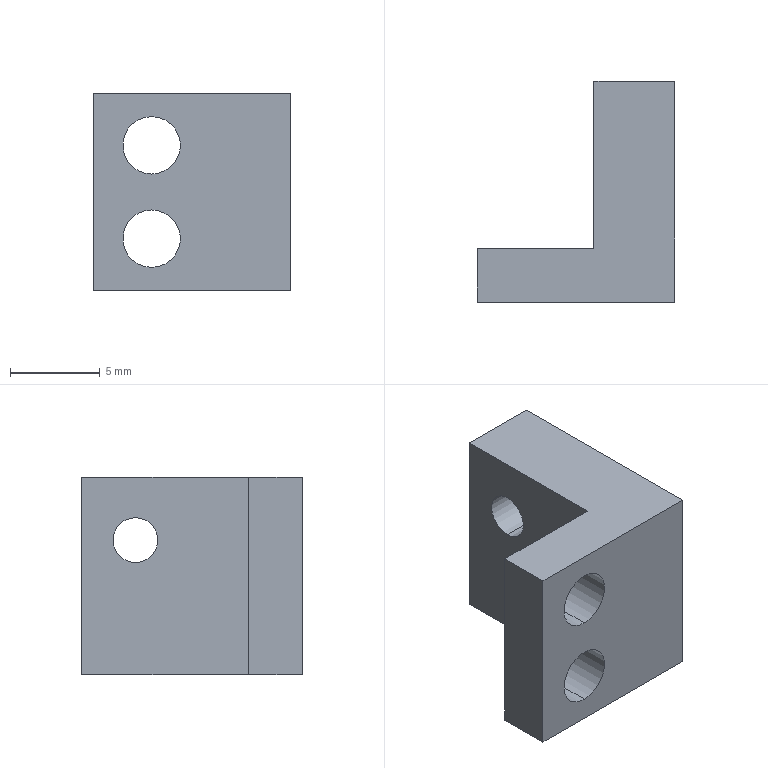Part | SolidWorks | features ICE 2, Chamfer 1, Extrusion 1, HoleWzd 1 | 1 solid | 18 faces | box 11 x 12.3 x 11 mm | volume 750.231 mm3 | plane 8 | cylinder 6 | cone 4 | commonest cylinder face diameters 3.2 x4 2.5 x2
STEP:
#1=CARTESIAN_POINT('',(-2.25,2.5,-4.2));
#2=VERTEX_POINT('',#1);
#3=CARTESIAN_POINT('',(-2.25,2.5,-1.));
#4=VERTEX_POINT('',#3);
#5=CARTESIAN_POINT('',(-2.25,2.5,-2.6));
#6=DIRECTION('',(0.,1.,0.));
#7=DIRECTION('',(0.,0.,1.));
#8=AXIS2_PLACEMENT_3D('',#5,#6,#7);
#9=CIRCLE('',#8,1.6);
#10=EDGE_CURVE('',#2,#4,#9,.T.);
#11=ORIENTED_EDGE('',*,*,#10,.F.);
#12=CARTESIAN_POINT('',(-2.25,3.,-4.7));
#13=VERTEX_POINT('',#12);
#14=CARTESIAN_POINT('',(-2.25,2.5,-4.2));
#15=DIRECTION('',(0.,0.7071,-0.7071));
#16=VECTOR('',#15,1000.);
#17=LINE('',#14,#16);
#18=EDGE_CURVE('',#2,#13,#17,.T.);
#19=ORIENTED_EDGE('',*,*,#18,.T.);
#20=CARTESIAN_POINT('',(-2.25,3.,-0.5));
#21=VERTEX_POINT('',#20);
#22=CARTESIAN_POINT('',(-2.25,3.,-2.6));
#23=DIRECTION('',(0.,-1.,0.));
#24=DIRECTION('',(0.,0.,1.));
#25=AXIS2_PLACEMENT_3D('',#22,#23,#24);
#26=CIRCLE('',#25,2.1);
#27=EDGE_CURVE('',#21,#13,#26,.T.);
#28=ORIENTED_EDGE('',*,*,#27,.F.);
#29=CARTESIAN_POINT('',(-2.25,2.5,-1.));
#30=DIRECTION('',(0.,0.7071,0.7071));
#31=VECTOR('',#30,1000.);
#32=LINE('',#29,#31);
#33=EDGE_CURVE('',#4,#21,#32,.T.);
#34=ORIENTED_EDGE('',*,*,#33,.F.);
#35=EDGE_LOOP('',(#11,#19,#28,#34));
#36=FACE_OUTER_BOUND('',#35,.T.);
#37=CARTESIAN_POINT('',(-2.25,2.5,-2.6));
#38=DIRECTION('',(0.,1.,0.));
#39=DIRECTION('',(0.,0.,1.));
#40=AXIS2_PLACEMENT_3D('',#37,#38,#39);
#41=CONICAL_SURFACE('',#40,1.6,0.7854);
#42=ADVANCED_FACE('',(#36),#41,.F.);
#43=CARTESIAN_POINT('',(-2.25,2.5,1.));
#44=VERTEX_POINT('',#43);
#45=CARTESIAN_POINT('',(-2.25,2.5,4.2));
#46=VERTEX_POINT('',#45);
#47=CARTESIAN_POINT('',(-2.25,2.5,2.6));
#48=DIRECTION('',(0.,1.,0.));
#49=DIRECTION('',(0.,0.,1.));
#50=AXIS2_PLACEMENT_3D('',#47,#48,#49);
#51=CIRCLE('',#50,1.6);
#52=EDGE_CURVE('',#44,#46,#51,.T.);
#53=ORIENTED_EDGE('',*,*,#52,.F.);
#54=CARTESIAN_POINT('',(-2.25,3.,0.5));
#55=VERTEX_POINT('',#54);
#56=CARTESIAN_POINT('',(-2.25,2.5,1.));
#57=DIRECTION('',(0.,0.7071,-0.7071));
#58=VECTOR('',#57,1000.);
#59=LINE('',#56,#58);
#60=EDGE_CURVE('',#44,#55,#59,.T.);
#61=ORIENTED_EDGE('',*,*,#60,.T.);
#62=CARTESIAN_POINT('',(-2.25,3.,4.7));
#63=VERTEX_POINT('',#62);
#64=CARTESIAN_POINT('',(-2.25,3.,2.6));
#65=DIRECTION('',(0.,-1.,0.));
#66=DIRECTION('',(0.,0.,1.));
#67=AXIS2_PLACEMENT_3D('',#64,#65,#66);
#68=CIRCLE('',#67,2.1);
#69=EDGE_CURVE('',#63,#55,#68,.T.);
#70=ORIENTED_EDGE('',*,*,#69,.F.);
#71=CARTESIAN_POINT('',(-2.25,2.5,4.2));
#72=DIRECTION('',(0.,0.7071,0.7071));
#73=VECTOR('',#72,1000.);
#74=LINE('',#71,#73);
#75=EDGE_CURVE('',#46,#63,#74,.T.);
#76=ORIENTED_EDGE('',*,*,#75,.F.);
#77=EDGE_LOOP('',(#53,#61,#70,#76));
#78=FACE_OUTER_BOUND('',#77,.T.);
#79=CARTESIAN_POINT('',(-2.25,2.5,2.6));
#80=DIRECTION('',(0.,1.,0.));
#81=DIRECTION('',(0.,0.,1.));
#82=AXIS2_PLACEMENT_3D('',#79,#80,#81);
#83=CONICAL_SURFACE('',#82,1.6,0.7854);
#84=ADVANCED_FACE('',(#78),#83,.F.);
#85=CARTESIAN_POINT('',(-2.25,0.,-4.2));
#86=VERTEX_POINT('',#85);
#87=CARTESIAN_POINT('',(-2.25,0.,-1.));
#88=VERTEX_POINT('',#87);
#89=CARTESIAN_POINT('',(-2.25,0.,-2.6));
#90=DIRECTION('',(0.,1.,0.));
#91=DIRECTION('',(0.,0.,1.));
#92=AXIS2_PLACEMENT_3D('',#89,#90,#91);
#93=CIRCLE('',#92,1.6);
#94=EDGE_CURVE('',#86,#88,#93,.T.);
#95=ORIENTED_EDGE('',*,*,#94,.F.);
#96=CARTESIAN_POINT('',(-2.25,0.,-4.2));
#97=DIRECTION('',(0.,1.,0.));
#98=VECTOR('',#97,1000.);
#99=LINE('',#96,#98);
#100=EDGE_CURVE('',#86,#2,#99,.T.);
#101=ORIENTED_EDGE('',*,*,#100,.T.);
#102=ORIENTED_EDGE('',*,*,#10,.T.);
#103=CARTESIAN_POINT('',(-2.25,0.,-1.));
#104=DIRECTION('',(0.,1.,0.));
#105=VECTOR('',#104,1000.);
#106=LINE('',#103,#105);
#107=EDGE_CURVE('',#88,#4,#106,.T.);
#108=ORIENTED_EDGE('',*,*,#107,.F.);
#109=EDGE_LOOP('',(#95,#101,#102,#108));
#110=FACE_OUTER_BOUND('',#109,.T.);
#111=CARTESIAN_POINT('',(-2.25,0.,-2.6));
#112=DIRECTION('',(0.,1.,0.));
#113=DIRECTION('',(0.,0.,1.));
#114=AXIS2_PLACEMENT_3D('',#111,#112,#113);
#115=CYLINDRICAL_SURFACE('',#114,1.6);
#116=ADVANCED_FACE('',(#110),#115,.F.);
#117=CARTESIAN_POINT('',(-2.25,0.,1.));
#118=VERTEX_POINT('',#117);
#119=CARTESIAN_POINT('',(-2.25,0.,4.2));
#120=VERTEX_POINT('',#119);
#121=CARTESIAN_POINT('',(-2.25,0.,2.6));
#122=DIRECTION('',(0.,1.,0.));
#123=DIRECTION('',(0.,0.,1.));
#124=AXIS2_PLACEMENT_3D('',#121,#122,#123);
#125=CIRCLE('',#124,1.6);
#126=EDGE_CURVE('',#118,#120,#125,.T.);
#127=ORIENTED_EDGE('',*,*,#126,.F.);
#128=CARTESIAN_POINT('',(-2.25,0.,1.));
#129=DIRECTION('',(0.,1.,0.));
#130=VECTOR('',#129,1000.);
#131=LINE('',#128,#130);
#132=EDGE_CURVE('',#118,#44,#131,.T.);
#133=ORIENTED_EDGE('',*,*,#132,.T.);
#134=ORIENTED_EDGE('',*,*,#52,.T.);
#135=CARTESIAN_POINT('',(-2.25,0.,4.2));
#136=DIRECTION('',(0.,1.,0.));
#137=VECTOR('',#136,1000.);
#138=LINE('',#135,#137);
#139=EDGE_CURVE('',#120,#46,#138,.T.);
#140=ORIENTED_EDGE('',*,*,#139,.F.);
#141=EDGE_LOOP('',(#127,#133,#134,#140));
#142=FACE_OUTER_BOUND('',#141,.T.);
#143=CARTESIAN_POINT('',(-2.25,0.,2.6));
#144=DIRECTION('',(0.,1.,0.));
#145=DIRECTION('',(0.,0.,1.));
#146=AXIS2_PLACEMENT_3D('',#143,#144,#145);
#147=CYLINDRICAL_SURFACE('',#146,1.6);
#148=ADVANCED_FACE('',(#142),#147,.F.);
#149=CARTESIAN_POINT('',(5.5,9.3,0.75));
#150=VERTEX_POINT('',#149);
#151=CARTESIAN_POINT('',(5.5,9.3,3.25));
#152=VERTEX_POINT('',#151);
#153=CARTESIAN_POINT('',(5.5,9.3,2.));
#154=DIRECTION('',(-1.,0.,0.));
#155=DIRECTION('',(0.,0.,1.));
#156=AXIS2_PLACEMENT_3D('',#153,#154,#155);
#157=CIRCLE('',#156,1.25);
#158=EDGE_CURVE('',#150,#152,#157,.T.);
#159=ORIENTED_EDGE('',*,*,#158,.F.);
#160=CARTESIAN_POINT('',(1.,9.3,0.75));
#161=VERTEX_POINT('',#160);
#162=CARTESIAN_POINT('',(1.,9.3,0.75));
#163=DIRECTION('',(-1.,0.,0.));
#164=VECTOR('',#163,1000.);
#165=LINE('',#162,#164);
#166=EDGE_CURVE('',#150,#161,#165,.T.);
#167=ORIENTED_EDGE('',*,*,#166,.T.);
#168=CARTESIAN_POINT('',(1.,9.3,3.25));
#169=VERTEX_POINT('',#168);
#170=CARTESIAN_POINT('',(1.,9.3,2.));
#171=DIRECTION('',(-1.,0.,0.));
#172=DIRECTION('',(0.,0.,1.));
#173=AXIS2_PLACEMENT_3D('',#170,#171,#172);
#174=CIRCLE('',#173,1.25);
#175=EDGE_CURVE('',#161,#169,#174,.T.);
#176=ORIENTED_EDGE('',*,*,#175,.T.);
#177=CARTESIAN_POINT('',(1.,9.3,3.25));
#178=DIRECTION('',(-1.,0.,0.));
#179=VECTOR('',#178,1000.);
#180=LINE('',#177,#179);
#181=EDGE_CURVE('',#152,#169,#180,.T.);
#182=ORIENTED_EDGE('',*,*,#181,.F.);
#183=EDGE_LOOP('',(#159,#167,#176,#182));
#184=FACE_OUTER_BOUND('',#183,.T.);
#185=CARTESIAN_POINT('',(1.,9.3,2.));
#186=DIRECTION('',(-1.,0.,0.));
#187=DIRECTION('',(0.,0.,1.));
#188=AXIS2_PLACEMENT_3D('',#185,#186,#187);
#189=CYLINDRICAL_SURFACE('',#188,1.25);
#190=ADVANCED_FACE('',(#184),#189,.F.);
#191=CARTESIAN_POINT('',(5.5,9.3,2.));
#192=DIRECTION('',(-1.,0.,0.));
#193=DIRECTION('',(0.,0.,1.));
#194=AXIS2_PLACEMENT_3D('',#191,#192,#193);
#195=CIRCLE('',#194,1.25);
#196=EDGE_CURVE('',#152,#150,#195,.T.);
#197=ORIENTED_EDGE('',*,*,#196,.T.);
#198=ORIENTED_EDGE('',*,*,#158,.T.);
#199=EDGE_LOOP('',(#197,#198));
#200=FACE_BOUND('',#199,.T.);
#201=CARTESIAN_POINT('',(5.5,0.,5.5));
#202=VERTEX_POINT('',#201);
#203=CARTESIAN_POINT('',(5.5,0.,-5.5));
#204=VERTEX_POINT('',#203);
#205=CARTESIAN_POINT('',(5.5,0.,-5.5));
#206=DIRECTION('',(0.,0.,-1.));
#207=VECTOR('',#206,1000.);
#208=LINE('',#205,#207);
#209=EDGE_CURVE('',#202,#204,#208,.T.);
#210=ORIENTED_EDGE('',*,*,#209,.T.);
#211=CARTESIAN_POINT('',(5.5,12.3,-5.5));
#212=VERTEX_POINT('',#211);
#213=CARTESIAN_POINT('',(5.5,3.,-5.5));
#214=DIRECTION('',(0.,-1.,0.));
#215=VECTOR('',#214,1000.);
#216=LINE('',#213,#215);
#217=EDGE_CURVE('',#212,#204,#216,.T.);
#218=ORIENTED_EDGE('',*,*,#217,.F.);
#219=CARTESIAN_POINT('',(5.5,12.3,5.5));
#220=VERTEX_POINT('',#219);
#221=CARTESIAN_POINT('',(5.5,12.3,-5.5));
#222=DIRECTION('',(0.,0.,-1.));
#223=VECTOR('',#222,1000.);
#224=LINE('',#221,#223);
#225=EDGE_CURVE('',#220,#212,#224,.T.);
#226=ORIENTED_EDGE('',*,*,#225,.F.);
#227=CARTESIAN_POINT('',(5.5,3.,5.5));
#228=DIRECTION('',(0.,-1.,0.));
#229=VECTOR('',#228,1000.);
#230=LINE('',#227,#229);
#231=EDGE_CURVE('',#220,#202,#230,.T.);
#232=ORIENTED_EDGE('',*,*,#231,.T.);
#233=EDGE_LOOP('',(#210,#218,#226,#232));
#234=FACE_OUTER_BOUND('',#233,.T.);
#235=CARTESIAN_POINT('',(5.5,3.,-5.5));
#236=DIRECTION('',(-1.,0.,0.));
#237=DIRECTION('',(0.,0.,1.));
#238=AXIS2_PLACEMENT_3D('',#235,#236,#237);
#239=PLANE('',#238);
#240=ADVANCED_FACE('',(#200,#234),#239,.F.);
#241=CARTESIAN_POINT('',(-5.5,0.,-5.5));
#242=VERTEX_POINT('',#241);
#243=CARTESIAN_POINT('',(-5.5,0.,-5.5));
#244=DIRECTION('',(-1.,0.,0.));
#245=VECTOR('',#244,1000.);
#246=LINE('',#243,#245);
#247=EDGE_CURVE('',#204,#242,#246,.T.);
#248=ORIENTED_EDGE('',*,*,#247,.T.);
#249=CARTESIAN_POINT('',(-5.5,3.,-5.5));
#250=VERTEX_POINT('',#249);
#251=CARTESIAN_POINT('',(-5.5,3.,-5.5));
#252=DIRECTION('',(0.,-1.,0.));
#253=VECTOR('',#252,1000.);
#254=LINE('',#251,#253);
#255=EDGE_CURVE('',#250,#242,#254,.T.);
#256=ORIENTED_EDGE('',*,*,#255,.F.);
#257=CARTESIAN_POINT('',(1.,3.,-5.5));
#258=VERTEX_POINT('',#257);
#259=CARTESIAN_POINT('',(-5.5,3.,-5.5));
#260=DIRECTION('',(-1.,0.,0.));
#261=VECTOR('',#260,1000.);
#262=LINE('',#259,#261);
#263=EDGE_CURVE('',#258,#250,#262,.T.);
#264=ORIENTED_EDGE('',*,*,#263,.F.);
#265=CARTESIAN_POINT('',(1.,12.3,-5.5));
#266=VERTEX_POINT('',#265);
#267=CARTESIAN_POINT('',(1.,12.3,-5.5));
#268=DIRECTION('',(0.,-1.,0.));
#269=VECTOR('',#268,1000.);
#270=LINE('',#267,#269);
#271=EDGE_CURVE('',#266,#258,#270,.T.);
#272=ORIENTED_EDGE('',*,*,#271,.F.);
#273=CARTESIAN_POINT('',(5.5,12.3,-5.5));
#274=DIRECTION('',(-1.,0.,0.));
#275=VECTOR('',#274,1000.);
#276=LINE('',#273,#275);
#277=EDGE_CURVE('',#212,#266,#276,.T.);
#278=ORIENTED_EDGE('',*,*,#277,.F.);
#279=ORIENTED_EDGE('',*,*,#217,.T.);
#280=EDGE_LOOP('',(#248,#256,#264,#272,#278,#279));
#281=FACE_OUTER_BOUND('',#280,.T.);
#282=CARTESIAN_POINT('',(-5.5,3.,-5.5));
#283=DIRECTION('',(0.,0.,1.));
#284=DIRECTION('',(1.,0.,0.));
#285=AXIS2_PLACEMENT_3D('',#282,#283,#284);
#286=PLANE('',#285);
#287=ADVANCED_FACE('',(#281),#286,.F.);
#288=CARTESIAN_POINT('',(-5.5,0.,5.5));
#289=VERTEX_POINT('',#288);
#290=CARTESIAN_POINT('',(-5.5,0.,-5.5));
#291=DIRECTION('',(0.,0.,1.));
#292=VECTOR('',#291,1000.);
#293=LINE('',#290,#292);
#294=EDGE_CURVE('',#242,#289,#293,.T.);
#295=ORIENTED_EDGE('',*,*,#294,.T.);
#296=CARTESIAN_POINT('',(-5.5,3.,5.5));
#297=VERTEX_POINT('',#296);
#298=CARTESIAN_POINT('',(-5.5,3.,5.5));
#299=DIRECTION('',(0.,-1.,0.));
#300=VECTOR('',#299,1000.);
#301=LINE('',#298,#300);
#302=EDGE_CURVE('',#297,#289,#301,.T.);
#303=ORIENTED_EDGE('',*,*,#302,.F.);
#304=CARTESIAN_POINT('',(-5.5,3.,-5.5));
#305=DIRECTION('',(0.,0.,1.));
#306=VECTOR('',#305,1000.);
#307=LINE('',#304,#306);
#308=EDGE_CURVE('',#250,#297,#307,.T.);
#309=ORIENTED_EDGE('',*,*,#308,.F.);
#310=ORIENTED_EDGE('',*,*,#255,.T.);
#311=EDGE_LOOP('',(#295,#303,#309,#310));
#312=FACE_OUTER_BOUND('',#311,.T.);
#313=CARTESIAN_POINT('',(-5.5,3.,-5.5));
#314=DIRECTION('',(1.,0.,0.));
#315=DIRECTION('',(0.,0.,-1.));
#316=AXIS2_PLACEMENT_3D('',#313,#314,#315);
#317=PLANE('',#316);
#318=ADVANCED_FACE('',(#312),#317,.F.);
#319=CARTESIAN_POINT('',(-5.5,0.,5.5));
#320=DIRECTION('',(1.,0.,0.));
#321=VECTOR('',#320,1000.);
#322=LINE('',#319,#321);
#323=EDGE_CURVE('',#289,#202,#322,.T.);
#324=ORIENTED_EDGE('',*,*,#323,.T.);
#325=ORIENTED_EDGE('',*,*,#231,.F.);
#326=CARTESIAN_POINT('',(1.,12.3,5.5));
#327=VERTEX_POINT('',#326);
#328=CARTESIAN_POINT('',(5.5,12.3,5.5));
#329=DIRECTION('',(1.,0.,0.));
#330=VECTOR('',#329,1000.);
#331=LINE('',#328,#330);
#332=EDGE_CURVE('',#327,#220,#331,.T.);
#333=ORIENTED_EDGE('',*,*,#332,.F.);
#334=CARTESIAN_POINT('',(1.,3.,5.5));
#335=VERTEX_POINT('',#334);
#336=CARTESIAN_POINT('',(1.,12.3,5.5));
#337=DIRECTION('',(0.,-1.,0.));
#338=VECTOR('',#337,1000.);
#339=LINE('',#336,#338);
#340=EDGE_CURVE('',#327,#335,#339,.T.);
#341=ORIENTED_EDGE('',*,*,#340,.T.);
#342=CARTESIAN_POINT('',(-5.5,3.,5.5));
#343=DIRECTION('',(1.,0.,0.));
#344=VECTOR('',#343,1000.);
#345=LINE('',#342,#344);
#346=EDGE_CURVE('',#297,#335,#345,.T.);
#347=ORIENTED_EDGE('',*,*,#346,.F.);
#348=ORIENTED_EDGE('',*,*,#302,.T.);
#349=EDGE_LOOP('',(#324,#325,#333,#341,#347,#348));
#350=FACE_OUTER_BOUND('',#349,.T.);
#351=CARTESIAN_POINT('',(-5.5,3.,5.5));
#352=DIRECTION('',(0.,0.,-1.));
#353=DIRECTION('',(-1.,0.,0.));
#354=AXIS2_PLACEMENT_3D('',#351,#352,#353);
#355=PLANE('',#354);
#356=ADVANCED_FACE('',(#350),#355,.F.);
#357=ORIENTED_EDGE('',*,*,#69,.T.);
#358=CARTESIAN_POINT('',(-2.25,3.,2.6));
#359=DIRECTION('',(0.,-1.,0.));
#360=DIRECTION('',(0.,0.,1.));
#361=AXIS2_PLACEMENT_3D('',#358,#359,#360);
#362=CIRCLE('',#361,2.1);
#363=EDGE_CURVE('',#55,#63,#362,.T.);
#364=ORIENTED_EDGE('',*,*,#363,.T.);
#365=EDGE_LOOP('',(#357,#364));
#366=FACE_BOUND('',#365,.T.);
#367=ORIENTED_EDGE('',*,*,#27,.T.);
#368=CARTESIAN_POINT('',(-2.25,3.,-2.6));
#369=DIRECTION('',(0.,-1.,0.));
#370=DIRECTION('',(0.,0.,1.));
#371=AXIS2_PLACEMENT_3D('',#368,#369,#370);
#372=CIRCLE('',#371,2.1);
#373=EDGE_CURVE('',#13,#21,#372,.T.);
#374=ORIENTED_EDGE('',*,*,#373,.T.);
#375=EDGE_LOOP('',(#367,#374));
#376=FACE_BOUND('',#375,.T.);
#377=CARTESIAN_POINT('',(1.,3.,-5.5));
#378=DIRECTION('',(0.,0.,1.));
#379=VECTOR('',#378,1000.);
#380=LINE('',#377,#379);
#381=EDGE_CURVE('',#258,#335,#380,.T.);
#382=ORIENTED_EDGE('',*,*,#381,.F.);
#383=ORIENTED_EDGE('',*,*,#263,.T.);
#384=ORIENTED_EDGE('',*,*,#308,.T.);
#385=ORIENTED_EDGE('',*,*,#346,.T.);
#386=EDGE_LOOP('',(#382,#383,#384,#385));
#387=FACE_OUTER_BOUND('',#386,.T.);
#388=CARTESIAN_POINT('',(0.,3.,0.));
#389=DIRECTION('',(0.,1.,0.));
#390=DIRECTION('',(0.,0.,1.));
#391=AXIS2_PLACEMENT_3D('',#388,#389,#390);
#392=PLANE('',#391);
#393=ADVANCED_FACE('',(#366,#376,#387),#392,.T.);
#394=CARTESIAN_POINT('',(-2.25,0.,-2.6));
#395=DIRECTION('',(0.,1.,0.));
#396=DIRECTION('',(0.,0.,1.));
#397=AXIS2_PLACEMENT_3D('',#394,#395,#396);
#398=CIRCLE('',#397,1.6);
#399=EDGE_CURVE('',#88,#86,#398,.T.);
#400=ORIENTED_EDGE('',*,*,#399,.T.);
#401=ORIENTED_EDGE('',*,*,#94,.T.);
#402=EDGE_LOOP('',(#400,#401));
#403=FACE_BOUND('',#402,.T.);
#404=CARTESIAN_POINT('',(-2.25,0.,2.6));
#405=DIRECTION('',(0.,1.,0.));
#406=DIRECTION('',(0.,0.,1.));
#407=AXIS2_PLACEMENT_3D('',#404,#405,#406);
#408=CIRCLE('',#407,1.6);
#409=EDGE_CURVE('',#120,#118,#408,.T.);
#410=ORIENTED_EDGE('',*,*,#409,.T.);
#411=ORIENTED_EDGE('',*,*,#126,.T.);
#412=EDGE_LOOP('',(#410,#411));
#413=FACE_BOUND('',#412,.T.);
#414=ORIENTED_EDGE('',*,*,#209,.F.);
#415=ORIENTED_EDGE('',*,*,#323,.F.);
#416=ORIENTED_EDGE('',*,*,#294,.F.);
#417=ORIENTED_EDGE('',*,*,#247,.F.);
#418=EDGE_LOOP('',(#414,#415,#416,#417));
#419=FACE_OUTER_BOUND('',#418,.T.);
#420=CARTESIAN_POINT('',(0.,0.,0.));
#421=DIRECTION('',(0.,1.,0.));
#422=DIRECTION('',(0.,0.,1.));
#423=AXIS2_PLACEMENT_3D('',#420,#421,#422);
#424=PLANE('',#423);
#425=ADVANCED_FACE('',(#403,#413,#419),#424,.F.);
#426=CARTESIAN_POINT('',(1.,9.3,2.));
#427=DIRECTION('',(-1.,0.,0.));
#428=DIRECTION('',(0.,0.,1.));
#429=AXIS2_PLACEMENT_3D('',#426,#427,#428);
#430=CIRCLE('',#429,1.25);
#431=EDGE_CURVE('',#169,#161,#430,.T.);
#432=ORIENTED_EDGE('',*,*,#431,.F.);
#433=ORIENTED_EDGE('',*,*,#175,.F.);
#434=EDGE_LOOP('',(#432,#433));
#435=FACE_BOUND('',#434,.T.);
#436=ORIENTED_EDGE('',*,*,#381,.T.);
#437=ORIENTED_EDGE('',*,*,#340,.F.);
#438=CARTESIAN_POINT('',(1.,12.3,-5.5));
#439=DIRECTION('',(0.,0.,1.));
#440=VECTOR('',#439,1000.);
#441=LINE('',#438,#440);
#442=EDGE_CURVE('',#266,#327,#441,.T.);
#443=ORIENTED_EDGE('',*,*,#442,.F.);
#444=ORIENTED_EDGE('',*,*,#271,.T.);
#445=EDGE_LOOP('',(#436,#437,#443,#444));
#446=FACE_OUTER_BOUND('',#445,.T.);
#447=CARTESIAN_POINT('',(1.,12.3,-5.5));
#448=DIRECTION('',(1.,0.,0.));
#449=DIRECTION('',(0.,0.,-1.));
#450=AXIS2_PLACEMENT_3D('',#447,#448,#449);
#451=PLANE('',#450);
#452=ADVANCED_FACE('',(#435,#446),#451,.F.);
#453=ORIENTED_EDGE('',*,*,#225,.T.);
#454=ORIENTED_EDGE('',*,*,#277,.T.);
#455=ORIENTED_EDGE('',*,*,#442,.T.);
#456=ORIENTED_EDGE('',*,*,#332,.T.);
#457=EDGE_LOOP('',(#453,#454,#455,#456));
#458=FACE_OUTER_BOUND('',#457,.T.);
#459=CARTESIAN_POINT('',(0.,12.3,0.));
#460=DIRECTION('',(0.,-1.,0.));
#461=DIRECTION('',(0.,0.,-1.));
#462=AXIS2_PLACEMENT_3D('',#459,#460,#461);
#463=PLANE('',#462);
#464=ADVANCED_FACE('',(#458),#463,.F.);
#465=ORIENTED_EDGE('',*,*,#166,.F.);
#466=ORIENTED_EDGE('',*,*,#196,.F.);
#467=ORIENTED_EDGE('',*,*,#181,.T.);
#468=ORIENTED_EDGE('',*,*,#431,.T.);
#469=EDGE_LOOP('',(#465,#466,#467,#468));
#470=FACE_OUTER_BOUND('',#469,.T.);
#471=CARTESIAN_POINT('',(1.,9.3,2.));
#472=DIRECTION('',(-1.,0.,0.));
#473=DIRECTION('',(0.,0.,1.));
#474=AXIS2_PLACEMENT_3D('',#471,#472,#473);
#475=CYLINDRICAL_SURFACE('',#474,1.25);
#476=ADVANCED_FACE('',(#470),#475,.F.);
#477=ORIENTED_EDGE('',*,*,#132,.F.);
#478=ORIENTED_EDGE('',*,*,#409,.F.);
#479=ORIENTED_EDGE('',*,*,#139,.T.);
#480=CARTESIAN_POINT('',(-2.25,2.5,2.6));
#481=DIRECTION('',(0.,1.,0.));
#482=DIRECTION('',(0.,0.,1.));
#483=AXIS2_PLACEMENT_3D('',#480,#481,#482);
#484=CIRCLE('',#483,1.6);
#485=EDGE_CURVE('',#46,#44,#484,.T.);
#486=ORIENTED_EDGE('',*,*,#485,.T.);
#487=EDGE_LOOP('',(#477,#478,#479,#486));
#488=FACE_OUTER_BOUND('',#487,.T.);
#489=CARTESIAN_POINT('',(-2.25,0.,2.6));
#490=DIRECTION('',(0.,1.,0.));
#491=DIRECTION('',(0.,0.,1.));
#492=AXIS2_PLACEMENT_3D('',#489,#490,#491);
#493=CYLINDRICAL_SURFACE('',#492,1.6);
#494=ADVANCED_FACE('',(#488),#493,.F.);
#495=ORIENTED_EDGE('',*,*,#100,.F.);
#496=ORIENTED_EDGE('',*,*,#399,.F.);
#497=ORIENTED_EDGE('',*,*,#107,.T.);
#498=CARTESIAN_POINT('',(-2.25,2.5,-2.6));
#499=DIRECTION('',(0.,1.,0.));
#500=DIRECTION('',(0.,0.,1.));
#501=AXIS2_PLACEMENT_3D('',#498,#499,#500);
#502=CIRCLE('',#501,1.6);
#503=EDGE_CURVE('',#4,#2,#502,.T.);
#504=ORIENTED_EDGE('',*,*,#503,.T.);
#505=EDGE_LOOP('',(#495,#496,#497,#504));
#506=FACE_OUTER_BOUND('',#505,.T.);
#507=CARTESIAN_POINT('',(-2.25,0.,-2.6));
#508=DIRECTION('',(0.,1.,0.));
#509=DIRECTION('',(0.,0.,1.));
#510=AXIS2_PLACEMENT_3D('',#507,#508,#509);
#511=CYLINDRICAL_SURFACE('',#510,1.6);
#512=ADVANCED_FACE('',(#506),#511,.F.);
#513=ORIENTED_EDGE('',*,*,#60,.F.);
#514=ORIENTED_EDGE('',*,*,#485,.F.);
#515=ORIENTED_EDGE('',*,*,#75,.T.);
#516=ORIENTED_EDGE('',*,*,#363,.F.);
#517=EDGE_LOOP('',(#513,#514,#515,#516));
#518=FACE_OUTER_BOUND('',#517,.T.);
#519=CARTESIAN_POINT('',(-2.25,2.5,2.6));
#520=DIRECTION('',(0.,1.,0.));
#521=DIRECTION('',(0.,0.,1.));
#522=AXIS2_PLACEMENT_3D('',#519,#520,#521);
#523=CONICAL_SURFACE('',#522,1.6,0.7854);
#524=ADVANCED_FACE('',(#518),#523,.F.);
#525=ORIENTED_EDGE('',*,*,#18,.F.);
#526=ORIENTED_EDGE('',*,*,#503,.F.);
#527=ORIENTED_EDGE('',*,*,#33,.T.);
#528=ORIENTED_EDGE('',*,*,#373,.F.);
#529=EDGE_LOOP('',(#525,#526,#527,#528));
#530=FACE_OUTER_BOUND('',#529,.T.);
#531=CARTESIAN_POINT('',(-2.25,2.5,-2.6));
#532=DIRECTION('',(0.,1.,0.));
#533=DIRECTION('',(0.,0.,1.));
#534=AXIS2_PLACEMENT_3D('',#531,#532,#533);
#535=CONICAL_SURFACE('',#534,1.6,0.7854);
#536=ADVANCED_FACE('',(#530),#535,.F.);
#537=CLOSED_SHELL('',(#42,#84,#116,#148,#190,#240,#287,#318,#356,#393,#425,#452,#464,#476,#494,#512,#524,#536));
#538=MANIFOLD_SOLID_BREP('',#537);
#539=CARTESIAN_POINT('',(0.,0.,0.));
#540=DIRECTION('',(0.,0.,1.));
#541=DIRECTION('',(1.,0.,0.));
#542=AXIS2_PLACEMENT_3D('',#539,#540,#541);
#543=(LENGTH_UNIT()NAMED_UNIT(*)SI_UNIT(.MILLI.,.METRE.));
#544=UNCERTAINTY_MEASURE_WITH_UNIT(LENGTH_MEASURE(0.00001),#543,'','');
#545=(NAMED_UNIT(*)PLANE_ANGLE_UNIT()SI_UNIT($,.RADIAN.));
#546=(NAMED_UNIT(*)SI_UNIT($,.STERADIAN.)SOLID_ANGLE_UNIT());
#547=(GEOMETRIC_REPRESENTATION_CONTEXT(3)GLOBAL_UNCERTAINTY_ASSIGNED_CONTEXT((#544))GLOBAL_UNIT_ASSIGNED_CONTEXT((#543,#545,#546))REPRESENTATION_CONTEXT('',''));
#548=ADVANCED_BREP_SHAPE_REPRESENTATION('',(#538,#542),#547);